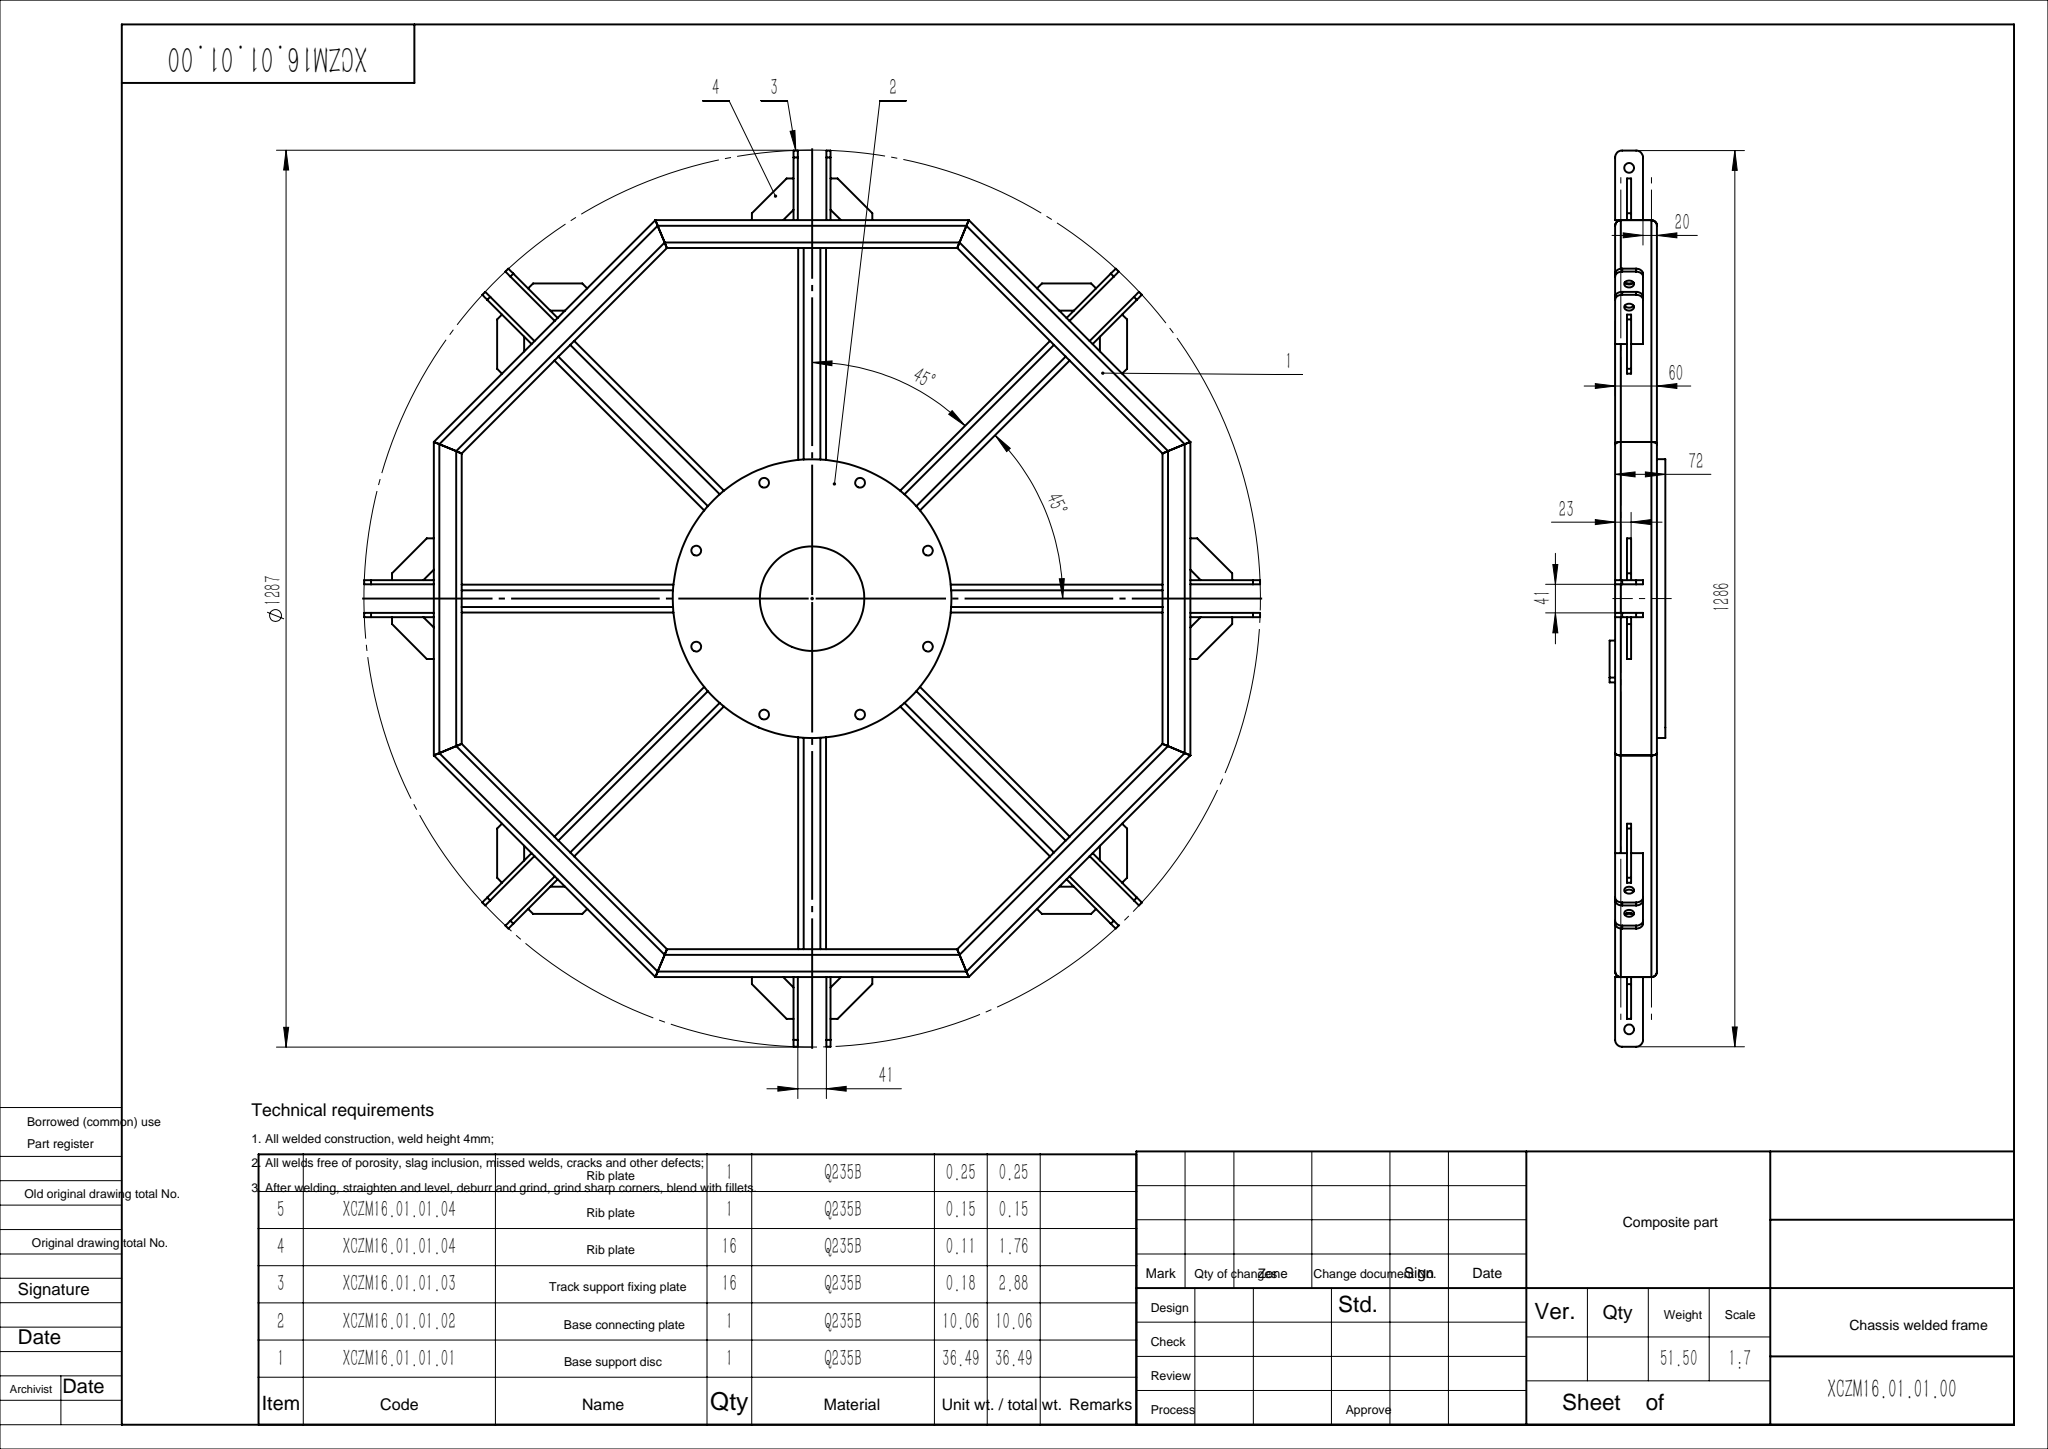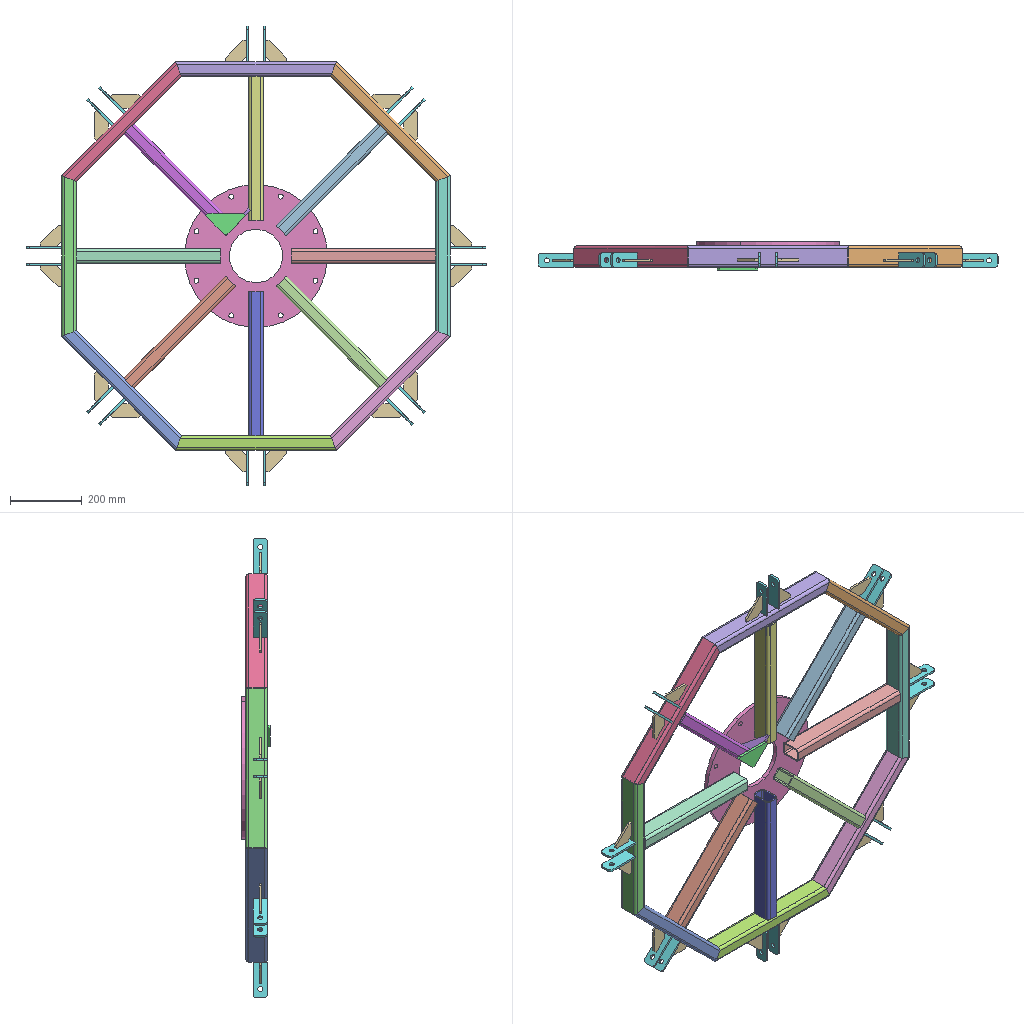Assembly | SolidWorks | 6 different items | 36 placed | box 1286 x 80 x 1286 mm
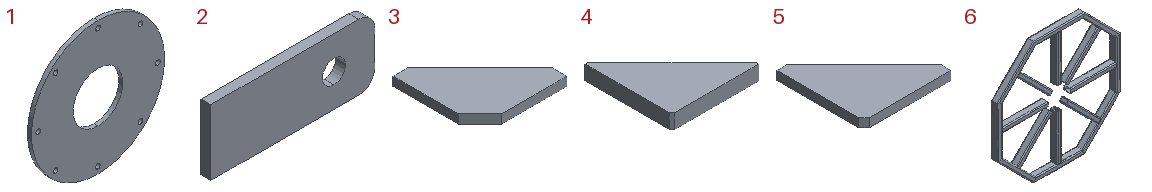Parts list (item | quantity | size | volume | features):
1 | x1 | 400 x 12 x 400 mm | 1281129 mm3 | features Extrusion 1, HoleWzd 1, RefAxis 1
2 | x16 | 100 x 6 x 40 mm | 22819 mm3 | features Extrusion 1
3 | x16 | 60 x 60 x 6 mm | 13425 mm3 | features Chamfer 1, Extrusion 1
4 | x1 | 60 x 60 x 10 mm | 19160 mm3 | features Chamfer 1, Extrusion 1
5 | x1 | 80 x 80 x 8 mm | 31500 mm3 | features Chamfer 1, Extrusion 1
6 | x1 | 1086 x 60 x 1086 mm | 4648285 mm3 | features WeldCornerFeat 8, CirPattern 1, RefAxis 1, WeldMemberFeat 1, WeldmentFeature 1
Mates (type | each side: item.copy, entity, surface, feature):
Coincident | 6.1 face plane CirPattern1 | 1.1 face plane Boss-Extrude1
PlanarAngleDim | 1.1 plane | assembly plane
Coincident | 6.1 axis | 1.1 axis
Coincident | 6.1 face plane Cold-formed hollow rectangular steel (GB/T 6728-2002) 60×40×4(1) | 2.1 face plane Boss-Extrude1 | 2 times
Concentric | 2.1 face cylinder Boss-Extrude1 | 2.2 face cylinder Boss-Extrude1
Parallel | 2.1 face plane Boss-Extrude1 | 2.2 face plane Boss-Extrude1
Width | 2.1 face plane Boss-Extrude1 | 2.2 face plane Boss-Extrude1 | 6.1 face plane CirPattern1 | 6.1 face plane CirPattern1
DistanceDim | 2.2 face plane Boss-Extrude1 | 2.1 face plane Boss-Extrude1
DistanceDim | 3.1 face plane Boss-Extrude1 | 6.1 face plane Cold-formed hollow rectangular steel (GB/T 6728-2002) 60×40×4(1)
Coincident | 6.1 face plane Cold-formed hollow rectangular steel (GB/T 6728-2002) 60×40×4(1) | 3.1 face plane Boss-Extrude1
Coincident | 3.1 face plane Boss-Extrude1 | 3.2 face plane Boss-Extrude1 | 2 times
Coincident | 3.1 face plane Boss-Extrude1 | 2.2 face plane Boss-Extrude1
Coincident | 2.1 face plane Boss-Extrude1 | 3.2 face plane Boss-Extrude1
Coincident | 4.1 face plane Boss-Extrude1 | 5.1 face plane Boss-Extrude1 | 2 times
Coincident | 6.1 face plane CirPattern1 | 4.1 face plane Boss-Extrude1 | 3 times
Coincident | 6.1 face plane CirPattern1 | 5.1 face plane Boss-Extrude1